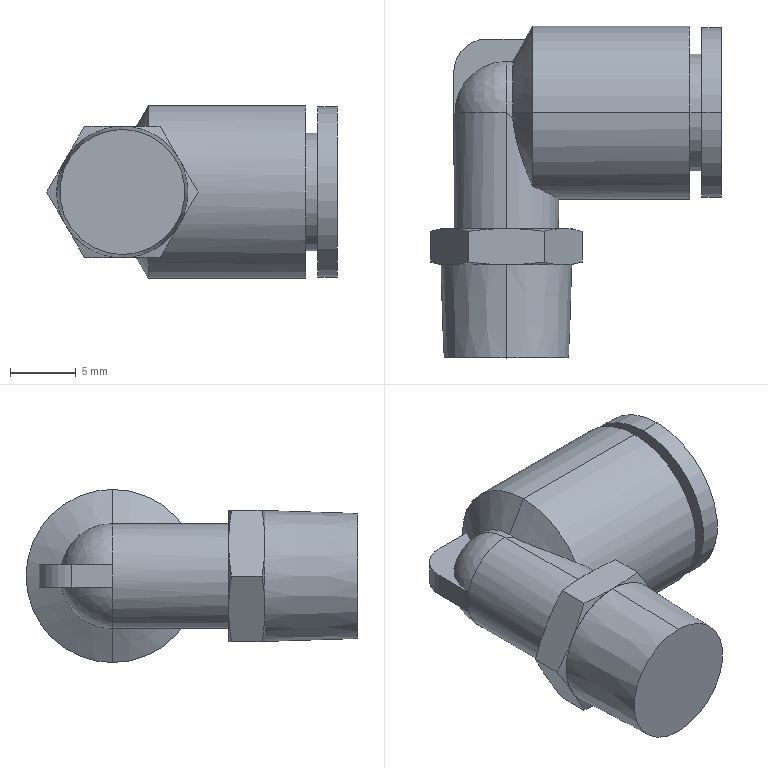Part | STEP file | 1 solid | 52 faces | box 22.174 x 25.3 x 13.2 mm | volume 2514 mm3 | plane 19 | cone 17 | cylinder 14 | spline 2 | commonest cylinder face diameters 8 x7 8.95 x2 13 x2 13.2 x2 5 x1